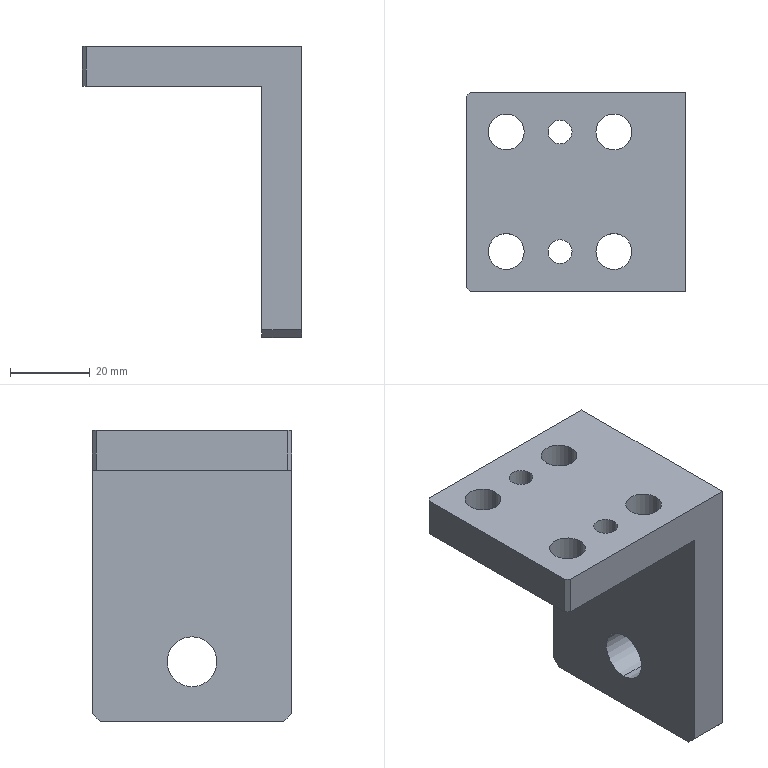Part | SolidWorks | features HoleWzd 3, Chamfer 2, Extrusion 1, ICE 1 | 1 solid | 26 faces | box 55 x 50 x 73 mm | volume 54613 mm3 | cylinder 14 | plane 12 | commonest cylinder face diameters 9 x8 6 x4 12.5 x2
STEP:
#1=CARTESIAN_POINT('',(-1.,-15.,10.));
#2=VERTEX_POINT('',#1);
#3=CARTESIAN_POINT('',(-7.,-15.,10.));
#4=VERTEX_POINT('',#3);
#5=CARTESIAN_POINT('',(-4.,-15.,10.));
#6=DIRECTION('',(0.,0.,-1.));
#7=DIRECTION('',(-1.,0.,0.));
#8=AXIS2_PLACEMENT_3D('',#5,#6,#7);
#9=CIRCLE('',#8,3.);
#10=EDGE_CURVE('',#2,#4,#9,.T.);
#11=ORIENTED_EDGE('',*,*,#10,.F.);
#12=CARTESIAN_POINT('',(-1.,-15.,0.));
#13=VERTEX_POINT('',#12);
#14=CARTESIAN_POINT('',(-1.,-15.,0.));
#15=DIRECTION('',(0.,0.,-1.));
#16=VECTOR('',#15,1000.);
#17=LINE('',#14,#16);
#18=EDGE_CURVE('',#2,#13,#17,.T.);
#19=ORIENTED_EDGE('',*,*,#18,.T.);
#20=CARTESIAN_POINT('',(-7.,-15.,0.));
#21=VERTEX_POINT('',#20);
#22=CARTESIAN_POINT('',(-4.,-15.,0.));
#23=DIRECTION('',(0.,0.,-1.));
#24=DIRECTION('',(-1.,0.,0.));
#25=AXIS2_PLACEMENT_3D('',#22,#23,#24);
#26=CIRCLE('',#25,3.);
#27=EDGE_CURVE('',#13,#21,#26,.T.);
#28=ORIENTED_EDGE('',*,*,#27,.T.);
#29=CARTESIAN_POINT('',(-7.,-15.,0.));
#30=DIRECTION('',(0.,0.,-1.));
#31=VECTOR('',#30,1000.);
#32=LINE('',#29,#31);
#33=EDGE_CURVE('',#4,#21,#32,.T.);
#34=ORIENTED_EDGE('',*,*,#33,.F.);
#35=EDGE_LOOP('',(#11,#19,#28,#34));
#36=FACE_OUTER_BOUND('',#35,.T.);
#37=CARTESIAN_POINT('',(-4.,-15.,0.));
#38=DIRECTION('',(0.,0.,-1.));
#39=DIRECTION('',(-1.,0.,0.));
#40=AXIS2_PLACEMENT_3D('',#37,#38,#39);
#41=CYLINDRICAL_SURFACE('',#40,3.);
#42=ADVANCED_FACE('',(#36),#41,.F.);
#43=CARTESIAN_POINT('',(-1.,15.,10.));
#44=VERTEX_POINT('',#43);
#45=CARTESIAN_POINT('',(-7.,15.,10.));
#46=VERTEX_POINT('',#45);
#47=CARTESIAN_POINT('',(-4.,15.,10.));
#48=DIRECTION('',(0.,0.,-1.));
#49=DIRECTION('',(-1.,0.,0.));
#50=AXIS2_PLACEMENT_3D('',#47,#48,#49);
#51=CIRCLE('',#50,3.);
#52=EDGE_CURVE('',#44,#46,#51,.T.);
#53=ORIENTED_EDGE('',*,*,#52,.F.);
#54=CARTESIAN_POINT('',(-1.,15.,0.));
#55=VERTEX_POINT('',#54);
#56=CARTESIAN_POINT('',(-1.,15.,0.));
#57=DIRECTION('',(0.,0.,-1.));
#58=VECTOR('',#57,1000.);
#59=LINE('',#56,#58);
#60=EDGE_CURVE('',#44,#55,#59,.T.);
#61=ORIENTED_EDGE('',*,*,#60,.T.);
#62=CARTESIAN_POINT('',(-7.,15.,0.));
#63=VERTEX_POINT('',#62);
#64=CARTESIAN_POINT('',(-4.,15.,0.));
#65=DIRECTION('',(0.,0.,-1.));
#66=DIRECTION('',(-1.,0.,0.));
#67=AXIS2_PLACEMENT_3D('',#64,#65,#66);
#68=CIRCLE('',#67,3.);
#69=EDGE_CURVE('',#55,#63,#68,.T.);
#70=ORIENTED_EDGE('',*,*,#69,.T.);
#71=CARTESIAN_POINT('',(-7.,15.,0.));
#72=DIRECTION('',(0.,0.,-1.));
#73=VECTOR('',#72,1000.);
#74=LINE('',#71,#73);
#75=EDGE_CURVE('',#46,#63,#74,.T.);
#76=ORIENTED_EDGE('',*,*,#75,.F.);
#77=EDGE_LOOP('',(#53,#61,#70,#76));
#78=FACE_OUTER_BOUND('',#77,.T.);
#79=CARTESIAN_POINT('',(-4.,15.,0.));
#80=DIRECTION('',(0.,0.,-1.));
#81=DIRECTION('',(-1.,0.,0.));
#82=AXIS2_PLACEMENT_3D('',#79,#80,#81);
#83=CYLINDRICAL_SURFACE('',#82,3.);
#84=ADVANCED_FACE('',(#78),#83,.F.);
#85=CARTESIAN_POINT('',(17.5,0.,-41.75));
#86=VERTEX_POINT('',#85);
#87=CARTESIAN_POINT('',(17.5,0.,-54.25));
#88=VERTEX_POINT('',#87);
#89=CARTESIAN_POINT('',(17.5,0.,-48.));
#90=DIRECTION('',(1.,0.,0.));
#91=DIRECTION('',(0.,1.,0.));
#92=AXIS2_PLACEMENT_3D('',#89,#90,#91);
#93=CIRCLE('',#92,6.25);
#94=EDGE_CURVE('',#86,#88,#93,.T.);
#95=ORIENTED_EDGE('',*,*,#94,.F.);
#96=CARTESIAN_POINT('',(27.5,0.,-41.75));
#97=VERTEX_POINT('',#96);
#98=CARTESIAN_POINT('',(27.5,0.,-41.75));
#99=DIRECTION('',(1.,0.,0.));
#100=VECTOR('',#99,1000.);
#101=LINE('',#98,#100);
#102=EDGE_CURVE('',#86,#97,#101,.T.);
#103=ORIENTED_EDGE('',*,*,#102,.T.);
#104=CARTESIAN_POINT('',(27.5,0.,-54.25));
#105=VERTEX_POINT('',#104);
#106=CARTESIAN_POINT('',(27.5,0.,-48.));
#107=DIRECTION('',(1.,0.,0.));
#108=DIRECTION('',(0.,0.,-1.));
#109=AXIS2_PLACEMENT_3D('',#106,#107,#108);
#110=CIRCLE('',#109,6.25);
#111=EDGE_CURVE('',#97,#105,#110,.T.);
#112=ORIENTED_EDGE('',*,*,#111,.T.);
#113=CARTESIAN_POINT('',(27.5,0.,-54.25));
#114=DIRECTION('',(1.,0.,0.));
#115=VECTOR('',#114,1000.);
#116=LINE('',#113,#115);
#117=EDGE_CURVE('',#88,#105,#116,.T.);
#118=ORIENTED_EDGE('',*,*,#117,.F.);
#119=EDGE_LOOP('',(#95,#103,#112,#118));
#120=FACE_OUTER_BOUND('',#119,.T.);
#121=CARTESIAN_POINT('',(27.5,0.,-48.));
#122=DIRECTION('',(1.,0.,0.));
#123=DIRECTION('',(0.,0.,-1.));
#124=AXIS2_PLACEMENT_3D('',#121,#122,#123);
#125=CYLINDRICAL_SURFACE('',#124,6.25);
#126=ADVANCED_FACE('',(#120),#125,.F.);
#127=CARTESIAN_POINT('',(-22.,-15.,10.));
#128=VERTEX_POINT('',#127);
#129=CARTESIAN_POINT('',(-13.,-15.,10.));
#130=VERTEX_POINT('',#129);
#131=CARTESIAN_POINT('',(-17.5,-15.,10.));
#132=DIRECTION('',(0.,0.,1.));
#133=DIRECTION('',(1.,0.,0.));
#134=AXIS2_PLACEMENT_3D('',#131,#132,#133);
#135=CIRCLE('',#134,4.5);
#136=EDGE_CURVE('',#128,#130,#135,.T.);
#137=ORIENTED_EDGE('',*,*,#136,.T.);
#138=CARTESIAN_POINT('',(-13.,-15.,0.));
#139=VERTEX_POINT('',#138);
#140=CARTESIAN_POINT('',(-13.,-15.,0.));
#141=DIRECTION('',(0.,0.,-1.));
#142=VECTOR('',#141,1000.);
#143=LINE('',#140,#142);
#144=EDGE_CURVE('',#130,#139,#143,.T.);
#145=ORIENTED_EDGE('',*,*,#144,.T.);
#146=CARTESIAN_POINT('',(-22.,-15.,0.));
#147=VERTEX_POINT('',#146);
#148=CARTESIAN_POINT('',(-17.5,-15.,0.));
#149=DIRECTION('',(0.,0.,-1.));
#150=DIRECTION('',(-1.,0.,0.));
#151=AXIS2_PLACEMENT_3D('',#148,#149,#150);
#152=CIRCLE('',#151,4.5);
#153=EDGE_CURVE('',#139,#147,#152,.T.);
#154=ORIENTED_EDGE('',*,*,#153,.T.);
#155=CARTESIAN_POINT('',(-22.,-15.,0.));
#156=DIRECTION('',(0.,0.,-1.));
#157=VECTOR('',#156,1000.);
#158=LINE('',#155,#157);
#159=EDGE_CURVE('',#128,#147,#158,.T.);
#160=ORIENTED_EDGE('',*,*,#159,.F.);
#161=EDGE_LOOP('',(#137,#145,#154,#160));
#162=FACE_OUTER_BOUND('',#161,.T.);
#163=CARTESIAN_POINT('',(-17.5,-15.,0.));
#164=DIRECTION('',(0.,0.,-1.));
#165=DIRECTION('',(-1.,0.,0.));
#166=AXIS2_PLACEMENT_3D('',#163,#164,#165);
#167=CYLINDRICAL_SURFACE('',#166,4.5);
#168=ADVANCED_FACE('',(#162),#167,.F.);
#169=CARTESIAN_POINT('',(-22.,15.,10.));
#170=VERTEX_POINT('',#169);
#171=CARTESIAN_POINT('',(-13.,15.,10.));
#172=VERTEX_POINT('',#171);
#173=CARTESIAN_POINT('',(-17.5,15.,10.));
#174=DIRECTION('',(0.,0.,1.));
#175=DIRECTION('',(1.,0.,0.));
#176=AXIS2_PLACEMENT_3D('',#173,#174,#175);
#177=CIRCLE('',#176,4.5);
#178=EDGE_CURVE('',#170,#172,#177,.T.);
#179=ORIENTED_EDGE('',*,*,#178,.T.);
#180=CARTESIAN_POINT('',(-13.,15.,0.));
#181=VERTEX_POINT('',#180);
#182=CARTESIAN_POINT('',(-13.,15.,0.));
#183=DIRECTION('',(0.,0.,-1.));
#184=VECTOR('',#183,1000.);
#185=LINE('',#182,#184);
#186=EDGE_CURVE('',#172,#181,#185,.T.);
#187=ORIENTED_EDGE('',*,*,#186,.T.);
#188=CARTESIAN_POINT('',(-22.,15.,0.));
#189=VERTEX_POINT('',#188);
#190=CARTESIAN_POINT('',(-17.5,15.,0.));
#191=DIRECTION('',(0.,0.,-1.));
#192=DIRECTION('',(-1.,0.,0.));
#193=AXIS2_PLACEMENT_3D('',#190,#191,#192);
#194=CIRCLE('',#193,4.5);
#195=EDGE_CURVE('',#181,#189,#194,.T.);
#196=ORIENTED_EDGE('',*,*,#195,.T.);
#197=CARTESIAN_POINT('',(-22.,15.,0.));
#198=DIRECTION('',(0.,0.,-1.));
#199=VECTOR('',#198,1000.);
#200=LINE('',#197,#199);
#201=EDGE_CURVE('',#170,#189,#200,.T.);
#202=ORIENTED_EDGE('',*,*,#201,.F.);
#203=EDGE_LOOP('',(#179,#187,#196,#202));
#204=FACE_OUTER_BOUND('',#203,.T.);
#205=CARTESIAN_POINT('',(-17.5,15.,0.));
#206=DIRECTION('',(0.,0.,-1.));
#207=DIRECTION('',(-1.,0.,0.));
#208=AXIS2_PLACEMENT_3D('',#205,#206,#207);
#209=CYLINDRICAL_SURFACE('',#208,4.5);
#210=ADVANCED_FACE('',(#204),#209,.F.);
#211=CARTESIAN_POINT('',(5.,-15.,10.));
#212=VERTEX_POINT('',#211);
#213=CARTESIAN_POINT('',(14.,-15.,10.));
#214=VERTEX_POINT('',#213);
#215=CARTESIAN_POINT('',(9.5,-15.,10.));
#216=DIRECTION('',(0.,0.,1.));
#217=DIRECTION('',(1.,0.,0.));
#218=AXIS2_PLACEMENT_3D('',#215,#216,#217);
#219=CIRCLE('',#218,4.5);
#220=EDGE_CURVE('',#212,#214,#219,.T.);
#221=ORIENTED_EDGE('',*,*,#220,.T.);
#222=CARTESIAN_POINT('',(14.,-15.,0.));
#223=VERTEX_POINT('',#222);
#224=CARTESIAN_POINT('',(14.,-15.,0.));
#225=DIRECTION('',(0.,0.,-1.));
#226=VECTOR('',#225,1000.);
#227=LINE('',#224,#226);
#228=EDGE_CURVE('',#214,#223,#227,.T.);
#229=ORIENTED_EDGE('',*,*,#228,.T.);
#230=CARTESIAN_POINT('',(5.,-15.,0.));
#231=VERTEX_POINT('',#230);
#232=CARTESIAN_POINT('',(9.5,-15.,0.));
#233=DIRECTION('',(0.,0.,-1.));
#234=DIRECTION('',(-1.,0.,0.));
#235=AXIS2_PLACEMENT_3D('',#232,#233,#234);
#236=CIRCLE('',#235,4.5);
#237=EDGE_CURVE('',#223,#231,#236,.T.);
#238=ORIENTED_EDGE('',*,*,#237,.T.);
#239=CARTESIAN_POINT('',(5.,-15.,0.));
#240=DIRECTION('',(0.,0.,-1.));
#241=VECTOR('',#240,1000.);
#242=LINE('',#239,#241);
#243=EDGE_CURVE('',#212,#231,#242,.T.);
#244=ORIENTED_EDGE('',*,*,#243,.F.);
#245=EDGE_LOOP('',(#221,#229,#238,#244));
#246=FACE_OUTER_BOUND('',#245,.T.);
#247=CARTESIAN_POINT('',(9.5,-15.,0.));
#248=DIRECTION('',(0.,0.,-1.));
#249=DIRECTION('',(-1.,0.,0.));
#250=AXIS2_PLACEMENT_3D('',#247,#248,#249);
#251=CYLINDRICAL_SURFACE('',#250,4.5);
#252=ADVANCED_FACE('',(#246),#251,.F.);
#253=CARTESIAN_POINT('',(5.,15.,10.));
#254=VERTEX_POINT('',#253);
#255=CARTESIAN_POINT('',(14.,15.,10.));
#256=VERTEX_POINT('',#255);
#257=CARTESIAN_POINT('',(9.5,15.,10.));
#258=DIRECTION('',(0.,0.,1.));
#259=DIRECTION('',(1.,0.,0.));
#260=AXIS2_PLACEMENT_3D('',#257,#258,#259);
#261=CIRCLE('',#260,4.5);
#262=EDGE_CURVE('',#254,#256,#261,.T.);
#263=ORIENTED_EDGE('',*,*,#262,.T.);
#264=CARTESIAN_POINT('',(14.,15.,0.));
#265=VERTEX_POINT('',#264);
#266=CARTESIAN_POINT('',(14.,15.,0.));
#267=DIRECTION('',(0.,0.,-1.));
#268=VECTOR('',#267,1000.);
#269=LINE('',#266,#268);
#270=EDGE_CURVE('',#256,#265,#269,.T.);
#271=ORIENTED_EDGE('',*,*,#270,.T.);
#272=CARTESIAN_POINT('',(5.,15.,0.));
#273=VERTEX_POINT('',#272);
#274=CARTESIAN_POINT('',(9.5,15.,0.));
#275=DIRECTION('',(0.,0.,-1.));
#276=DIRECTION('',(-1.,0.,0.));
#277=AXIS2_PLACEMENT_3D('',#274,#275,#276);
#278=CIRCLE('',#277,4.5);
#279=EDGE_CURVE('',#265,#273,#278,.T.);
#280=ORIENTED_EDGE('',*,*,#279,.T.);
#281=CARTESIAN_POINT('',(5.,15.,0.));
#282=DIRECTION('',(0.,0.,-1.));
#283=VECTOR('',#282,1000.);
#284=LINE('',#281,#283);
#285=EDGE_CURVE('',#254,#273,#284,.T.);
#286=ORIENTED_EDGE('',*,*,#285,.F.);
#287=EDGE_LOOP('',(#263,#271,#280,#286));
#288=FACE_OUTER_BOUND('',#287,.T.);
#289=CARTESIAN_POINT('',(9.5,15.,0.));
#290=DIRECTION('',(0.,0.,-1.));
#291=DIRECTION('',(-1.,0.,0.));
#292=AXIS2_PLACEMENT_3D('',#289,#290,#291);
#293=CYLINDRICAL_SURFACE('',#292,4.5);
#294=ADVANCED_FACE('',(#288),#293,.F.);
#295=CARTESIAN_POINT('',(-4.,-15.,0.));
#296=DIRECTION('',(0.,0.,-1.));
#297=DIRECTION('',(-1.,0.,0.));
#298=AXIS2_PLACEMENT_3D('',#295,#296,#297);
#299=CIRCLE('',#298,3.);
#300=EDGE_CURVE('',#21,#13,#299,.T.);
#301=ORIENTED_EDGE('',*,*,#300,.F.);
#302=ORIENTED_EDGE('',*,*,#27,.F.);
#303=EDGE_LOOP('',(#301,#302));
#304=FACE_BOUND('',#303,.T.);
#305=CARTESIAN_POINT('',(-4.,15.,0.));
#306=DIRECTION('',(0.,0.,-1.));
#307=DIRECTION('',(-1.,0.,0.));
#308=AXIS2_PLACEMENT_3D('',#305,#306,#307);
#309=CIRCLE('',#308,3.);
#310=EDGE_CURVE('',#63,#55,#309,.T.);
#311=ORIENTED_EDGE('',*,*,#310,.F.);
#312=ORIENTED_EDGE('',*,*,#69,.F.);
#313=EDGE_LOOP('',(#311,#312));
#314=FACE_BOUND('',#313,.T.);
#315=CARTESIAN_POINT('',(-17.5,-15.,0.));
#316=DIRECTION('',(0.,0.,-1.));
#317=DIRECTION('',(-1.,0.,0.));
#318=AXIS2_PLACEMENT_3D('',#315,#316,#317);
#319=CIRCLE('',#318,4.5);
#320=EDGE_CURVE('',#147,#139,#319,.T.);
#321=ORIENTED_EDGE('',*,*,#320,.F.);
#322=ORIENTED_EDGE('',*,*,#153,.F.);
#323=EDGE_LOOP('',(#321,#322));
#324=FACE_BOUND('',#323,.T.);
#325=CARTESIAN_POINT('',(-17.5,15.,0.));
#326=DIRECTION('',(0.,0.,-1.));
#327=DIRECTION('',(-1.,0.,0.));
#328=AXIS2_PLACEMENT_3D('',#325,#326,#327);
#329=CIRCLE('',#328,4.5);
#330=EDGE_CURVE('',#189,#181,#329,.T.);
#331=ORIENTED_EDGE('',*,*,#330,.F.);
#332=ORIENTED_EDGE('',*,*,#195,.F.);
#333=EDGE_LOOP('',(#331,#332));
#334=FACE_BOUND('',#333,.T.);
#335=CARTESIAN_POINT('',(9.5,-15.,0.));
#336=DIRECTION('',(0.,0.,-1.));
#337=DIRECTION('',(-1.,0.,0.));
#338=AXIS2_PLACEMENT_3D('',#335,#336,#337);
#339=CIRCLE('',#338,4.5);
#340=EDGE_CURVE('',#231,#223,#339,.T.);
#341=ORIENTED_EDGE('',*,*,#340,.F.);
#342=ORIENTED_EDGE('',*,*,#237,.F.);
#343=EDGE_LOOP('',(#341,#342));
#344=FACE_BOUND('',#343,.T.);
#345=CARTESIAN_POINT('',(9.5,15.,0.));
#346=DIRECTION('',(0.,0.,-1.));
#347=DIRECTION('',(-1.,0.,0.));
#348=AXIS2_PLACEMENT_3D('',#345,#346,#347);
#349=CIRCLE('',#348,4.5);
#350=EDGE_CURVE('',#273,#265,#349,.T.);
#351=ORIENTED_EDGE('',*,*,#350,.F.);
#352=ORIENTED_EDGE('',*,*,#279,.F.);
#353=EDGE_LOOP('',(#351,#352));
#354=FACE_BOUND('',#353,.T.);
#355=CARTESIAN_POINT('',(-26.5,-25.,0.));
#356=VERTEX_POINT('',#355);
#357=CARTESIAN_POINT('',(17.5,-25.,0.));
#358=VERTEX_POINT('',#357);
#359=CARTESIAN_POINT('',(-27.5,-25.,0.));
#360=DIRECTION('',(1.,0.,0.));
#361=VECTOR('',#360,1000.);
#362=LINE('',#359,#361);
#363=EDGE_CURVE('',#356,#358,#362,.T.);
#364=ORIENTED_EDGE('',*,*,#363,.F.);
#365=CARTESIAN_POINT('',(-27.5,-24.,0.));
#366=VERTEX_POINT('',#365);
#367=CARTESIAN_POINT('',(-26.5,-25.,0.));
#368=DIRECTION('',(-0.7071,0.7071,0.));
#369=VECTOR('',#368,1000.);
#370=LINE('',#367,#369);
#371=EDGE_CURVE('',#356,#366,#370,.T.);
#372=ORIENTED_EDGE('',*,*,#371,.T.);
#373=CARTESIAN_POINT('',(-27.5,24.,0.));
#374=VERTEX_POINT('',#373);
#375=CARTESIAN_POINT('',(-27.5,25.,0.));
#376=DIRECTION('',(0.,-1.,0.));
#377=VECTOR('',#376,1000.);
#378=LINE('',#375,#377);
#379=EDGE_CURVE('',#374,#366,#378,.T.);
#380=ORIENTED_EDGE('',*,*,#379,.F.);
#381=CARTESIAN_POINT('',(-26.5,25.,0.));
#382=VERTEX_POINT('',#381);
#383=CARTESIAN_POINT('',(-27.5,24.,0.));
#384=DIRECTION('',(0.7071,0.7071,0.));
#385=VECTOR('',#384,1000.);
#386=LINE('',#383,#385);
#387=EDGE_CURVE('',#374,#382,#386,.T.);
#388=ORIENTED_EDGE('',*,*,#387,.T.);
#389=CARTESIAN_POINT('',(17.5,25.,0.));
#390=VERTEX_POINT('',#389);
#391=CARTESIAN_POINT('',(-27.5,25.,0.));
#392=DIRECTION('',(-1.,0.,0.));
#393=VECTOR('',#392,1000.);
#394=LINE('',#391,#393);
#395=EDGE_CURVE('',#390,#382,#394,.T.);
#396=ORIENTED_EDGE('',*,*,#395,.F.);
#397=CARTESIAN_POINT('',(17.5,25.,0.));
#398=DIRECTION('',(0.,1.,0.));
#399=VECTOR('',#398,1000.);
#400=LINE('',#397,#399);
#401=EDGE_CURVE('',#358,#390,#400,.T.);
#402=ORIENTED_EDGE('',*,*,#401,.F.);
#403=EDGE_LOOP('',(#364,#372,#380,#388,#396,#402));
#404=FACE_OUTER_BOUND('',#403,.T.);
#405=CARTESIAN_POINT('',(0.,0.,0.));
#406=DIRECTION('',(0.,0.,1.));
#407=DIRECTION('',(1.,0.,0.));
#408=AXIS2_PLACEMENT_3D('',#405,#406,#407);
#409=PLANE('',#408);
#410=ADVANCED_FACE('',(#304,#314,#324,#334,#344,#354,#404),#409,.F.);
#411=CARTESIAN_POINT('',(27.5,0.,-48.));
#412=DIRECTION('',(1.,0.,0.));
#413=DIRECTION('',(0.,0.,-1.));
#414=AXIS2_PLACEMENT_3D('',#411,#412,#413);
#415=CIRCLE('',#414,6.25);
#416=EDGE_CURVE('',#105,#97,#415,.T.);
#417=ORIENTED_EDGE('',*,*,#416,.F.);
#418=ORIENTED_EDGE('',*,*,#111,.F.);
#419=EDGE_LOOP('',(#417,#418));
#420=FACE_BOUND('',#419,.T.);
#421=CARTESIAN_POINT('',(27.5,23.,-63.));
#422=VERTEX_POINT('',#421);
#423=CARTESIAN_POINT('',(27.5,-23.,-63.));
#424=VERTEX_POINT('',#423);
#425=CARTESIAN_POINT('',(27.5,25.,-63.));
#426=DIRECTION('',(0.,-1.,0.));
#427=VECTOR('',#426,1000.);
#428=LINE('',#425,#427);
#429=EDGE_CURVE('',#422,#424,#428,.T.);
#430=ORIENTED_EDGE('',*,*,#429,.F.);
#431=CARTESIAN_POINT('',(27.5,25.,-61.));
#432=VERTEX_POINT('',#431);
#433=CARTESIAN_POINT('',(27.5,23.,-63.));
#434=DIRECTION('',(0.,0.7071,0.7071));
#435=VECTOR('',#434,1000.);
#436=LINE('',#433,#435);
#437=EDGE_CURVE('',#422,#432,#436,.T.);
#438=ORIENTED_EDGE('',*,*,#437,.T.);
#439=CARTESIAN_POINT('',(27.5,25.,10.));
#440=VERTEX_POINT('',#439);
#441=CARTESIAN_POINT('',(27.5,25.,10.));
#442=DIRECTION('',(0.,0.,-1.));
#443=VECTOR('',#442,1000.);
#444=LINE('',#441,#443);
#445=EDGE_CURVE('',#440,#432,#444,.T.);
#446=ORIENTED_EDGE('',*,*,#445,.F.);
#447=CARTESIAN_POINT('',(27.5,-25.,10.));
#448=VERTEX_POINT('',#447);
#449=CARTESIAN_POINT('',(27.5,25.,10.));
#450=DIRECTION('',(0.,1.,0.));
#451=VECTOR('',#450,1000.);
#452=LINE('',#449,#451);
#453=EDGE_CURVE('',#448,#440,#452,.T.);
#454=ORIENTED_EDGE('',*,*,#453,.F.);
#455=CARTESIAN_POINT('',(27.5,-25.,-61.));
#456=VERTEX_POINT('',#455);
#457=CARTESIAN_POINT('',(27.5,-25.,10.));
#458=DIRECTION('',(0.,0.,-1.));
#459=VECTOR('',#458,1000.);
#460=LINE('',#457,#459);
#461=EDGE_CURVE('',#448,#456,#460,.T.);
#462=ORIENTED_EDGE('',*,*,#461,.T.);
#463=CARTESIAN_POINT('',(27.5,-23.,-63.));
#464=DIRECTION('',(0.,0.7071,-0.7071));
#465=VECTOR('',#464,1000.);
#466=LINE('',#463,#465);
#467=EDGE_CURVE('',#456,#424,#466,.T.);
#468=ORIENTED_EDGE('',*,*,#467,.T.);
#469=EDGE_LOOP('',(#430,#438,#446,#454,#462,#468));
#470=FACE_OUTER_BOUND('',#469,.T.);
#471=CARTESIAN_POINT('',(27.5,25.,10.));
#472=DIRECTION('',(-1.,0.,0.));
#473=DIRECTION('',(0.,-1.,0.));
#474=AXIS2_PLACEMENT_3D('',#471,#472,#473);
#475=PLANE('',#474);
#476=ADVANCED_FACE('',(#420,#470),#475,.F.);
#477=ORIENTED_EDGE('',*,*,#445,.T.);
#478=CARTESIAN_POINT('',(17.5,25.,-61.));
#479=VERTEX_POINT('',#478);
#480=CARTESIAN_POINT('',(-27.5,25.,-61.));
#481=DIRECTION('',(-1.,0.,0.));
#482=VECTOR('',#481,1000.);
#483=LINE('',#480,#482);
#484=EDGE_CURVE('',#432,#479,#483,.T.);
#485=ORIENTED_EDGE('',*,*,#484,.T.);
#486=CARTESIAN_POINT('',(17.5,25.,-63.));
#487=DIRECTION('',(0.,0.,1.));
#488=VECTOR('',#487,1000.);
#489=LINE('',#486,#488);
#490=EDGE_CURVE('',#479,#390,#489,.T.);
#491=ORIENTED_EDGE('',*,*,#490,.T.);
#492=ORIENTED_EDGE('',*,*,#395,.T.);
#493=CARTESIAN_POINT('',(-26.5,25.,10.));
#494=VERTEX_POINT('',#493);
#495=CARTESIAN_POINT('',(-26.5,25.,10.));
#496=DIRECTION('',(0.,0.,1.));
#497=VECTOR('',#496,1000.);
#498=LINE('',#495,#497);
#499=EDGE_CURVE('',#382,#494,#498,.T.);
#500=ORIENTED_EDGE('',*,*,#499,.T.);
#501=CARTESIAN_POINT('',(-27.5,25.,10.));
#502=DIRECTION('',(-1.,0.,0.));
#503=VECTOR('',#502,1000.);
#504=LINE('',#501,#503);
#505=EDGE_CURVE('',#440,#494,#504,.T.);
#506=ORIENTED_EDGE('',*,*,#505,.F.);
#507=EDGE_LOOP('',(#477,#485,#491,#492,#500,#506));
#508=FACE_OUTER_BOUND('',#507,.T.);
#509=CARTESIAN_POINT('',(-27.5,25.,10.));
#510=DIRECTION('',(0.,-1.,0.));
#511=DIRECTION('',(0.,0.,-1.));
#512=AXIS2_PLACEMENT_3D('',#509,#510,#511);
#513=PLANE('',#512);
#514=ADVANCED_FACE('',(#508),#513,.F.);
#515=ORIENTED_EDGE('',*,*,#379,.T.);
#516=CARTESIAN_POINT('',(-27.5,-24.,10.));
#517=VERTEX_POINT('',#516);
#518=CARTESIAN_POINT('',(-27.5,-24.,10.));
#519=DIRECTION('',(0.,0.,1.));
#520=VECTOR('',#519,1000.);
#521=LINE('',#518,#520);
#522=EDGE_CURVE('',#366,#517,#521,.T.);
#523=ORIENTED_EDGE('',*,*,#522,.T.);
#524=CARTESIAN_POINT('',(-27.5,24.,10.));
#525=VERTEX_POINT('',#524);
#526=CARTESIAN_POINT('',(-27.5,25.,10.));
#527=DIRECTION('',(0.,-1.,0.));
#528=VECTOR('',#527,1000.);
#529=LINE('',#526,#528);
#530=EDGE_CURVE('',#525,#517,#529,.T.);
#531=ORIENTED_EDGE('',*,*,#530,.F.);
#532=CARTESIAN_POINT('',(-27.5,24.,10.));
#533=DIRECTION('',(0.,0.,-1.));
#534=VECTOR('',#533,1000.);
#535=LINE('',#532,#534);
#536=EDGE_CURVE('',#525,#374,#535,.T.);
#537=ORIENTED_EDGE('',*,*,#536,.T.);
#538=EDGE_LOOP('',(#515,#523,#531,#537));
#539=FACE_OUTER_BOUND('',#538,.T.);
#540=CARTESIAN_POINT('',(-27.5,25.,10.));
#541=DIRECTION('',(1.,0.,0.));
#542=DIRECTION('',(0.,1.,0.));
#543=AXIS2_PLACEMENT_3D('',#540,#541,#542);
#544=PLANE('',#543);
#545=ADVANCED_FACE('',(#539),#544,.F.);
#546=CARTESIAN_POINT('',(17.5,-25.,-61.));
#547=VERTEX_POINT('',#546);
#548=CARTESIAN_POINT('',(17.5,-25.,-63.));
#549=DIRECTION('',(0.,0.,1.));
#550=VECTOR('',#549,1000.);
#551=LINE('',#548,#550);
#552=EDGE_CURVE('',#547,#358,#551,.T.);
#553=ORIENTED_EDGE('',*,*,#552,.F.);
#554=CARTESIAN_POINT('',(-27.5,-25.,-61.));
#555=DIRECTION('',(1.,0.,0.));
#556=VECTOR('',#555,1000.);
#557=LINE('',#554,#556);
#558=EDGE_CURVE('',#547,#456,#557,.T.);
#559=ORIENTED_EDGE('',*,*,#558,.T.);
#560=ORIENTED_EDGE('',*,*,#461,.F.);
#561=CARTESIAN_POINT('',(-26.5,-25.,10.));
#562=VERTEX_POINT('',#561);
#563=CARTESIAN_POINT('',(-27.5,-25.,10.));
#564=DIRECTION('',(1.,0.,0.));
#565=VECTOR('',#564,1000.);
#566=LINE('',#563,#565);
#567=EDGE_CURVE('',#562,#448,#566,.T.);
#568=ORIENTED_EDGE('',*,*,#567,.F.);
#569=CARTESIAN_POINT('',(-26.5,-25.,10.));
#570=DIRECTION('',(0.,0.,-1.));
#571=VECTOR('',#570,1000.);
#572=LINE('',#569,#571);
#573=EDGE_CURVE('',#562,#356,#572,.T.);
#574=ORIENTED_EDGE('',*,*,#573,.T.);
#575=ORIENTED_EDGE('',*,*,#363,.T.);
#576=EDGE_LOOP('',(#553,#559,#560,#568,#574,#575));
#577=FACE_OUTER_BOUND('',#576,.T.);
#578=CARTESIAN_POINT('',(-27.5,-25.,10.));
#579=DIRECTION('',(0.,1.,0.));
#580=DIRECTION('',(0.,0.,1.));
#581=AXIS2_PLACEMENT_3D('',#578,#579,#580);
#582=PLANE('',#581);
#583=ADVANCED_FACE('',(#577),#582,.F.);
#584=CARTESIAN_POINT('',(-4.,-15.,10.));
#585=DIRECTION('',(0.,0.,-1.));
#586=DIRECTION('',(-1.,0.,0.));
#587=AXIS2_PLACEMENT_3D('',#584,#585,#586);
#588=CIRCLE('',#587,3.);
#589=EDGE_CURVE('',#4,#2,#588,.T.);
#590=ORIENTED_EDGE('',*,*,#589,.T.);
#591=ORIENTED_EDGE('',*,*,#10,.T.);
#592=EDGE_LOOP('',(#590,#591));
#593=FACE_BOUND('',#592,.T.);
#594=CARTESIAN_POINT('',(-4.,15.,10.));
#595=DIRECTION('',(0.,0.,-1.));
#596=DIRECTION('',(-1.,0.,0.));
#597=AXIS2_PLACEMENT_3D('',#594,#595,#596);
#598=CIRCLE('',#597,3.);
#599=EDGE_CURVE('',#46,#44,#598,.T.);
#600=ORIENTED_EDGE('',*,*,#599,.T.);
#601=ORIENTED_EDGE('',*,*,#52,.T.);
#602=EDGE_LOOP('',(#600,#601));
#603=FACE_BOUND('',#602,.T.);
#604=ORIENTED_EDGE('',*,*,#136,.F.);
#605=CARTESIAN_POINT('',(-17.5,-15.,10.));
#606=DIRECTION('',(0.,0.,1.));
#607=DIRECTION('',(1.,0.,0.));
#608=AXIS2_PLACEMENT_3D('',#605,#606,#607);
#609=CIRCLE('',#608,4.5);
#610=EDGE_CURVE('',#130,#128,#609,.T.);
#611=ORIENTED_EDGE('',*,*,#610,.F.);
#612=EDGE_LOOP('',(#604,#611));
#613=FACE_BOUND('',#612,.T.);
#614=ORIENTED_EDGE('',*,*,#178,.F.);
#615=CARTESIAN_POINT('',(-17.5,15.,10.));
#616=DIRECTION('',(0.,0.,1.));
#617=DIRECTION('',(1.,0.,0.));
#618=AXIS2_PLACEMENT_3D('',#615,#616,#617);
#619=CIRCLE('',#618,4.5);
#620=EDGE_CURVE('',#172,#170,#619,.T.);
#621=ORIENTED_EDGE('',*,*,#620,.F.);
#622=EDGE_LOOP('',(#614,#621));
#623=FACE_BOUND('',#622,.T.);
#624=ORIENTED_EDGE('',*,*,#220,.F.);
#625=CARTESIAN_POINT('',(9.5,-15.,10.));
#626=DIRECTION('',(0.,0.,1.));
#627=DIRECTION('',(1.,0.,0.));
#628=AXIS2_PLACEMENT_3D('',#625,#626,#627);
#629=CIRCLE('',#628,4.5);
#630=EDGE_CURVE('',#214,#212,#629,.T.);
#631=ORIENTED_EDGE('',*,*,#630,.F.);
#632=EDGE_LOOP('',(#624,#631));
#633=FACE_BOUND('',#632,.T.);
#634=ORIENTED_EDGE('',*,*,#262,.F.);
#635=CARTESIAN_POINT('',(9.5,15.,10.));
#636=DIRECTION('',(0.,0.,1.));
#637=DIRECTION('',(1.,0.,0.));
#638=AXIS2_PLACEMENT_3D('',#635,#636,#637);
#639=CIRCLE('',#638,4.5);
#640=EDGE_CURVE('',#256,#254,#639,.T.);
#641=ORIENTED_EDGE('',*,*,#640,.F.);
#642=EDGE_LOOP('',(#634,#641));
#643=FACE_BOUND('',#642,.T.);
#644=ORIENTED_EDGE('',*,*,#530,.T.);
#645=CARTESIAN_POINT('',(-25.75,-25.75,10.));
#646=DIRECTION('',(0.7071,-0.7071,0.));
#647=VECTOR('',#646,1000.);
#648=LINE('',#645,#647);
#649=EDGE_CURVE('',#517,#562,#648,.T.);
#650=ORIENTED_EDGE('',*,*,#649,.T.);
#651=ORIENTED_EDGE('',*,*,#567,.T.);
#652=ORIENTED_EDGE('',*,*,#453,.T.);
#653=ORIENTED_EDGE('',*,*,#505,.T.);
#654=CARTESIAN_POINT('',(-25.75,25.75,10.));
#655=DIRECTION('',(-0.7071,-0.7071,0.));
#656=VECTOR('',#655,1000.);
#657=LINE('',#654,#656);
#658=EDGE_CURVE('',#494,#525,#657,.T.);
#659=ORIENTED_EDGE('',*,*,#658,.T.);
#660=EDGE_LOOP('',(#644,#650,#651,#652,#653,#659));
#661=FACE_OUTER_BOUND('',#660,.T.);
#662=CARTESIAN_POINT('',(0.,0.,10.));
#663=DIRECTION('',(0.,0.,1.));
#664=DIRECTION('',(1.,0.,0.));
#665=AXIS2_PLACEMENT_3D('',#662,#663,#664);
#666=PLANE('',#665);
#667=ADVANCED_FACE('',(#593,#603,#613,#623,#633,#643,#661),#666,.T.);
#668=CARTESIAN_POINT('',(17.5,0.,-48.));
#669=DIRECTION('',(1.,0.,0.));
#670=DIRECTION('',(0.,1.,0.));
#671=AXIS2_PLACEMENT_3D('',#668,#669,#670);
#672=CIRCLE('',#671,6.25);
#673=EDGE_CURVE('',#88,#86,#672,.T.);
#674=ORIENTED_EDGE('',*,*,#673,.T.);
#675=ORIENTED_EDGE('',*,*,#94,.T.);
#676=EDGE_LOOP('',(#674,#675));
#677=FACE_BOUND('',#676,.T.);
#678=ORIENTED_EDGE('',*,*,#490,.F.);
#679=CARTESIAN_POINT('',(17.5,23.,-63.));
#680=VERTEX_POINT('',#679);
#681=CARTESIAN_POINT('',(17.5,23.,-63.));
#682=DIRECTION('',(0.,-0.7071,-0.7071));
#683=VECTOR('',#682,1000.);
#684=LINE('',#681,#683);
#685=EDGE_CURVE('',#479,#680,#684,.T.);
#686=ORIENTED_EDGE('',*,*,#685,.T.);
#687=CARTESIAN_POINT('',(17.5,-23.,-63.));
#688=VERTEX_POINT('',#687);
#689=CARTESIAN_POINT('',(17.5,25.,-63.));
#690=DIRECTION('',(0.,1.,0.));
#691=VECTOR('',#690,1000.);
#692=LINE('',#689,#691);
#693=EDGE_CURVE('',#688,#680,#692,.T.);
#694=ORIENTED_EDGE('',*,*,#693,.F.);
#695=CARTESIAN_POINT('',(17.5,-23.,-63.));
#696=DIRECTION('',(0.,-0.7071,0.7071));
#697=VECTOR('',#696,1000.);
#698=LINE('',#695,#697);
#699=EDGE_CURVE('',#688,#547,#698,.T.);
#700=ORIENTED_EDGE('',*,*,#699,.T.);
#701=ORIENTED_EDGE('',*,*,#552,.T.);
#702=ORIENTED_EDGE('',*,*,#401,.T.);
#703=EDGE_LOOP('',(#678,#686,#694,#700,#701,#702));
#704=FACE_OUTER_BOUND('',#703,.T.);
#705=CARTESIAN_POINT('',(17.5,25.,-63.));
#706=DIRECTION('',(1.,0.,0.));
#707=DIRECTION('',(0.,1.,0.));
#708=AXIS2_PLACEMENT_3D('',#705,#706,#707);
#709=PLANE('',#708);
#710=ADVANCED_FACE('',(#677,#704),#709,.F.);
#711=ORIENTED_EDGE('',*,*,#693,.T.);
#712=CARTESIAN_POINT('',(0.,23.,-63.));
#713=DIRECTION('',(1.,0.,0.));
#714=VECTOR('',#713,1000.);
#715=LINE('',#712,#714);
#716=EDGE_CURVE('',#680,#422,#715,.T.);
#717=ORIENTED_EDGE('',*,*,#716,.T.);
#718=ORIENTED_EDGE('',*,*,#429,.T.);
#719=CARTESIAN_POINT('',(0.,-23.,-63.));
#720=DIRECTION('',(-1.,0.,0.));
#721=VECTOR('',#720,1000.);
#722=LINE('',#719,#721);
#723=EDGE_CURVE('',#424,#688,#722,.T.);
#724=ORIENTED_EDGE('',*,*,#723,.T.);
#725=EDGE_LOOP('',(#711,#717,#718,#724));
#726=FACE_OUTER_BOUND('',#725,.T.);
#727=CARTESIAN_POINT('',(0.,0.,-63.));
#728=DIRECTION('',(0.,0.,1.));
#729=DIRECTION('',(1.,0.,0.));
#730=AXIS2_PLACEMENT_3D('',#727,#728,#729);
#731=PLANE('',#730);
#732=ADVANCED_FACE('',(#726),#731,.F.);
#733=ORIENTED_EDGE('',*,*,#270,.F.);
#734=ORIENTED_EDGE('',*,*,#640,.T.);
#735=ORIENTED_EDGE('',*,*,#285,.T.);
#736=ORIENTED_EDGE('',*,*,#350,.T.);
#737=EDGE_LOOP('',(#733,#734,#735,#736));
#738=FACE_OUTER_BOUND('',#737,.T.);
#739=CARTESIAN_POINT('',(9.5,15.,0.));
#740=DIRECTION('',(0.,0.,-1.));
#741=DIRECTION('',(-1.,0.,0.));
#742=AXIS2_PLACEMENT_3D('',#739,#740,#741);
#743=CYLINDRICAL_SURFACE('',#742,4.5);
#744=ADVANCED_FACE('',(#738),#743,.F.);
#745=ORIENTED_EDGE('',*,*,#228,.F.);
#746=ORIENTED_EDGE('',*,*,#630,.T.);
#747=ORIENTED_EDGE('',*,*,#243,.T.);
#748=ORIENTED_EDGE('',*,*,#340,.T.);
#749=EDGE_LOOP('',(#745,#746,#747,#748));
#750=FACE_OUTER_BOUND('',#749,.T.);
#751=CARTESIAN_POINT('',(9.5,-15.,0.));
#752=DIRECTION('',(0.,0.,-1.));
#753=DIRECTION('',(-1.,0.,0.));
#754=AXIS2_PLACEMENT_3D('',#751,#752,#753);
#755=CYLINDRICAL_SURFACE('',#754,4.5);
#756=ADVANCED_FACE('',(#750),#755,.F.);
#757=ORIENTED_EDGE('',*,*,#186,.F.);
#758=ORIENTED_EDGE('',*,*,#620,.T.);
#759=ORIENTED_EDGE('',*,*,#201,.T.);
#760=ORIENTED_EDGE('',*,*,#330,.T.);
#761=EDGE_LOOP('',(#757,#758,#759,#760));
#762=FACE_OUTER_BOUND('',#761,.T.);
#763=CARTESIAN_POINT('',(-17.5,15.,0.));
#764=DIRECTION('',(0.,0.,-1.));
#765=DIRECTION('',(-1.,0.,0.));
#766=AXIS2_PLACEMENT_3D('',#763,#764,#765);
#767=CYLINDRICAL_SURFACE('',#766,4.5);
#768=ADVANCED_FACE('',(#762),#767,.F.);
#769=ORIENTED_EDGE('',*,*,#144,.F.);
#770=ORIENTED_EDGE('',*,*,#610,.T.);
#771=ORIENTED_EDGE('',*,*,#159,.T.);
#772=ORIENTED_EDGE('',*,*,#320,.T.);
#773=EDGE_LOOP('',(#769,#770,#771,#772));
#774=FACE_OUTER_BOUND('',#773,.T.);
#775=CARTESIAN_POINT('',(-17.5,-15.,0.));
#776=DIRECTION('',(0.,0.,-1.));
#777=DIRECTION('',(-1.,0.,0.));
#778=AXIS2_PLACEMENT_3D('',#775,#776,#777);
#779=CYLINDRICAL_SURFACE('',#778,4.5);
#780=ADVANCED_FACE('',(#774),#779,.F.);
#781=ORIENTED_EDGE('',*,*,#649,.F.);
#782=ORIENTED_EDGE('',*,*,#522,.F.);
#783=ORIENTED_EDGE('',*,*,#371,.F.);
#784=ORIENTED_EDGE('',*,*,#573,.F.);
#785=EDGE_LOOP('',(#781,#782,#783,#784));
#786=FACE_OUTER_BOUND('',#785,.T.);
#787=CARTESIAN_POINT('',(-26.5,-25.,10.));
#788=DIRECTION('',(0.7071,0.7071,0.));
#789=DIRECTION('',(0.,0.,-1.));
#790=AXIS2_PLACEMENT_3D('',#787,#788,#789);
#791=PLANE('',#790);
#792=ADVANCED_FACE('',(#786),#791,.F.);
#793=ORIENTED_EDGE('',*,*,#658,.F.);
#794=ORIENTED_EDGE('',*,*,#499,.F.);
#795=ORIENTED_EDGE('',*,*,#387,.F.);
#796=ORIENTED_EDGE('',*,*,#536,.F.);
#797=EDGE_LOOP('',(#793,#794,#795,#796));
#798=FACE_OUTER_BOUND('',#797,.T.);
#799=CARTESIAN_POINT('',(-27.5,24.,10.));
#800=DIRECTION('',(0.7071,-0.7071,0.));
#801=DIRECTION('',(0.,0.,-1.));
#802=AXIS2_PLACEMENT_3D('',#799,#800,#801);
#803=PLANE('',#802);
#804=ADVANCED_FACE('',(#798),#803,.F.);
#805=ORIENTED_EDGE('',*,*,#102,.F.);
#806=ORIENTED_EDGE('',*,*,#673,.F.);
#807=ORIENTED_EDGE('',*,*,#117,.T.);
#808=ORIENTED_EDGE('',*,*,#416,.T.);
#809=EDGE_LOOP('',(#805,#806,#807,#808));
#810=FACE_OUTER_BOUND('',#809,.T.);
#811=CARTESIAN_POINT('',(27.5,0.,-48.));
#812=DIRECTION('',(1.,0.,0.));
#813=DIRECTION('',(0.,0.,-1.));
#814=AXIS2_PLACEMENT_3D('',#811,#812,#813);
#815=CYLINDRICAL_SURFACE('',#814,6.25);
#816=ADVANCED_FACE('',(#810),#815,.F.);
#817=ORIENTED_EDGE('',*,*,#685,.F.);
#818=ORIENTED_EDGE('',*,*,#484,.F.);
#819=ORIENTED_EDGE('',*,*,#437,.F.);
#820=ORIENTED_EDGE('',*,*,#716,.F.);
#821=EDGE_LOOP('',(#817,#818,#819,#820));
#822=FACE_OUTER_BOUND('',#821,.T.);
#823=CARTESIAN_POINT('',(0.,23.,-63.));
#824=DIRECTION('',(0.,-0.7071,0.7071));
#825=DIRECTION('',(1.,0.,0.));
#826=AXIS2_PLACEMENT_3D('',#823,#824,#825);
#827=PLANE('',#826);
#828=ADVANCED_FACE('',(#822),#827,.F.);
#829=ORIENTED_EDGE('',*,*,#467,.F.);
#830=ORIENTED_EDGE('',*,*,#558,.F.);
#831=ORIENTED_EDGE('',*,*,#699,.F.);
#832=ORIENTED_EDGE('',*,*,#723,.F.);
#833=EDGE_LOOP('',(#829,#830,#831,#832));
#834=FACE_OUTER_BOUND('',#833,.T.);
#835=CARTESIAN_POINT('',(0.,-23.,-63.));
#836=DIRECTION('',(0.,0.7071,0.7071));
#837=DIRECTION('',(-1.,0.,0.));
#838=AXIS2_PLACEMENT_3D('',#835,#836,#837);
#839=PLANE('',#838);
#840=ADVANCED_FACE('',(#834),#839,.F.);
#841=ORIENTED_EDGE('',*,*,#60,.F.);
#842=ORIENTED_EDGE('',*,*,#599,.F.);
#843=ORIENTED_EDGE('',*,*,#75,.T.);
#844=ORIENTED_EDGE('',*,*,#310,.T.);
#845=EDGE_LOOP('',(#841,#842,#843,#844));
#846=FACE_OUTER_BOUND('',#845,.T.);
#847=CARTESIAN_POINT('',(-4.,15.,0.));
#848=DIRECTION('',(0.,0.,-1.));
#849=DIRECTION('',(-1.,0.,0.));
#850=AXIS2_PLACEMENT_3D('',#847,#848,#849);
#851=CYLINDRICAL_SURFACE('',#850,3.);
#852=ADVANCED_FACE('',(#846),#851,.F.);
#853=ORIENTED_EDGE('',*,*,#18,.F.);
#854=ORIENTED_EDGE('',*,*,#589,.F.);
#855=ORIENTED_EDGE('',*,*,#33,.T.);
#856=ORIENTED_EDGE('',*,*,#300,.T.);
#857=EDGE_LOOP('',(#853,#854,#855,#856));
#858=FACE_OUTER_BOUND('',#857,.T.);
#859=CARTESIAN_POINT('',(-4.,-15.,0.));
#860=DIRECTION('',(0.,0.,-1.));
#861=DIRECTION('',(-1.,0.,0.));
#862=AXIS2_PLACEMENT_3D('',#859,#860,#861);
#863=CYLINDRICAL_SURFACE('',#862,3.);
#864=ADVANCED_FACE('',(#858),#863,.F.);
#865=CLOSED_SHELL('',(#42,#84,#126,#168,#210,#252,#294,#410,#476,#514,#545,#583,#667,#710,#732,#744,#756,#768,#780,#792,#804,#816,#828,#840,#852,#864));
#866=MANIFOLD_SOLID_BREP('',#865);
#867=CARTESIAN_POINT('',(0.,0.,0.));
#868=DIRECTION('',(0.,0.,1.));
#869=DIRECTION('',(1.,0.,0.));
#870=AXIS2_PLACEMENT_3D('',#867,#868,#869);
#871=(LENGTH_UNIT()NAMED_UNIT(*)SI_UNIT(.MILLI.,.METRE.));
#872=UNCERTAINTY_MEASURE_WITH_UNIT(LENGTH_MEASURE(0.00001),#871,'','');
#873=(NAMED_UNIT(*)PLANE_ANGLE_UNIT()SI_UNIT($,.RADIAN.));
#874=(NAMED_UNIT(*)SI_UNIT($,.STERADIAN.)SOLID_ANGLE_UNIT());
#875=(GEOMETRIC_REPRESENTATION_CONTEXT(3)GLOBAL_UNCERTAINTY_ASSIGNED_CONTEXT((#872))GLOBAL_UNIT_ASSIGNED_CONTEXT((#871,#873,#874))REPRESENTATION_CONTEXT('',''));
#876=ADVANCED_BREP_SHAPE_REPRESENTATION('',(#866,#870),#875);